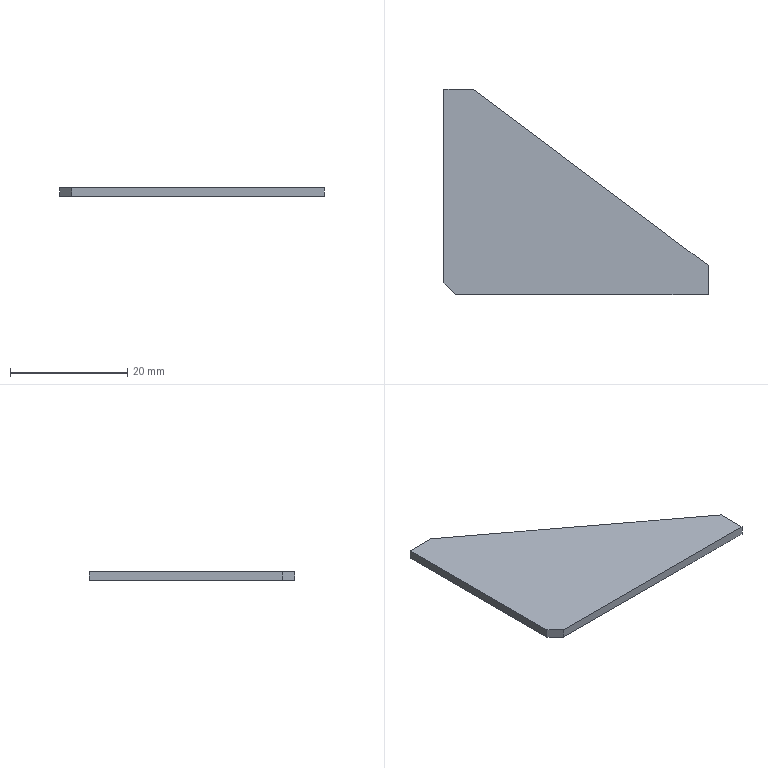Part | SolidWorks | features Extrusion 1 | 1 solid | 8 faces | box 45 x 35 x 1.5 mm | volume 1460 mm3 | plane 8
STEP:
#1=CARTESIAN_POINT('',(-20.5,-17.5,0.));
#2=VERTEX_POINT('',#1);
#3=CARTESIAN_POINT('',(22.5,-17.5,0.));
#4=VERTEX_POINT('',#3);
#5=CARTESIAN_POINT('',(22.5,-17.5,0.));
#6=DIRECTION('',(1.,0.,0.));
#7=VECTOR('',#6,1000.);
#8=LINE('',#5,#7);
#9=EDGE_CURVE('',#2,#4,#8,.T.);
#10=ORIENTED_EDGE('',*,*,#9,.T.);
#11=CARTESIAN_POINT('',(22.5,-17.5,1.5));
#12=VERTEX_POINT('',#11);
#13=CARTESIAN_POINT('',(22.5,-17.5,1.5));
#14=DIRECTION('',(0.,0.,-1.));
#15=VECTOR('',#14,1000.);
#16=LINE('',#13,#15);
#17=EDGE_CURVE('',#12,#4,#16,.T.);
#18=ORIENTED_EDGE('',*,*,#17,.F.);
#19=CARTESIAN_POINT('',(-20.5,-17.5,1.5));
#20=VERTEX_POINT('',#19);
#21=CARTESIAN_POINT('',(22.5,-17.5,1.5));
#22=DIRECTION('',(1.,0.,0.));
#23=VECTOR('',#22,1000.);
#24=LINE('',#21,#23);
#25=EDGE_CURVE('',#20,#12,#24,.T.);
#26=ORIENTED_EDGE('',*,*,#25,.F.);
#27=CARTESIAN_POINT('',(-20.5,-17.5,1.5));
#28=DIRECTION('',(0.,0.,-1.));
#29=VECTOR('',#28,1000.);
#30=LINE('',#27,#29);
#31=EDGE_CURVE('',#20,#2,#30,.T.);
#32=ORIENTED_EDGE('',*,*,#31,.T.);
#33=EDGE_LOOP('',(#10,#18,#26,#32));
#34=FACE_OUTER_BOUND('',#33,.T.);
#35=CARTESIAN_POINT('',(22.5,-17.5,1.5));
#36=DIRECTION('',(0.,1.,0.));
#37=DIRECTION('',(-1.,0.,0.));
#38=AXIS2_PLACEMENT_3D('',#35,#36,#37);
#39=PLANE('',#38);
#40=ADVANCED_FACE('',(#34),#39,.F.);
#41=CARTESIAN_POINT('',(22.5,-12.5,0.));
#42=VERTEX_POINT('',#41);
#43=CARTESIAN_POINT('',(22.5,-12.5,0.));
#44=DIRECTION('',(0.,1.,0.));
#45=VECTOR('',#44,1000.);
#46=LINE('',#43,#45);
#47=EDGE_CURVE('',#4,#42,#46,.T.);
#48=ORIENTED_EDGE('',*,*,#47,.T.);
#49=CARTESIAN_POINT('',(22.5,-12.5,1.5));
#50=VERTEX_POINT('',#49);
#51=CARTESIAN_POINT('',(22.5,-12.5,1.5));
#52=DIRECTION('',(0.,0.,-1.));
#53=VECTOR('',#52,1000.);
#54=LINE('',#51,#53);
#55=EDGE_CURVE('',#50,#42,#54,.T.);
#56=ORIENTED_EDGE('',*,*,#55,.F.);
#57=CARTESIAN_POINT('',(22.5,-12.5,1.5));
#58=DIRECTION('',(0.,1.,0.));
#59=VECTOR('',#58,1000.);
#60=LINE('',#57,#59);
#61=EDGE_CURVE('',#12,#50,#60,.T.);
#62=ORIENTED_EDGE('',*,*,#61,.F.);
#63=ORIENTED_EDGE('',*,*,#17,.T.);
#64=EDGE_LOOP('',(#48,#56,#62,#63));
#65=FACE_OUTER_BOUND('',#64,.T.);
#66=CARTESIAN_POINT('',(22.5,-12.5,1.5));
#67=DIRECTION('',(-1.,0.,0.));
#68=DIRECTION('',(0.,0.,1.));
#69=AXIS2_PLACEMENT_3D('',#66,#67,#68);
#70=PLANE('',#69);
#71=ADVANCED_FACE('',(#65),#70,.F.);
#72=CARTESIAN_POINT('',(-17.5,17.5,0.));
#73=VERTEX_POINT('',#72);
#74=CARTESIAN_POINT('',(-17.5,17.5,0.));
#75=DIRECTION('',(-0.8,0.6,0.));
#76=VECTOR('',#75,1000.);
#77=LINE('',#74,#76);
#78=EDGE_CURVE('',#42,#73,#77,.T.);
#79=ORIENTED_EDGE('',*,*,#78,.T.);
#80=CARTESIAN_POINT('',(-17.5,17.5,1.5));
#81=VERTEX_POINT('',#80);
#82=CARTESIAN_POINT('',(-17.5,17.5,1.5));
#83=DIRECTION('',(0.,0.,-1.));
#84=VECTOR('',#83,1000.);
#85=LINE('',#82,#84);
#86=EDGE_CURVE('',#81,#73,#85,.T.);
#87=ORIENTED_EDGE('',*,*,#86,.F.);
#88=CARTESIAN_POINT('',(-17.5,17.5,1.5));
#89=DIRECTION('',(-0.8,0.6,0.));
#90=VECTOR('',#89,1000.);
#91=LINE('',#88,#90);
#92=EDGE_CURVE('',#50,#81,#91,.T.);
#93=ORIENTED_EDGE('',*,*,#92,.F.);
#94=ORIENTED_EDGE('',*,*,#55,.T.);
#95=EDGE_LOOP('',(#79,#87,#93,#94));
#96=FACE_OUTER_BOUND('',#95,.T.);
#97=CARTESIAN_POINT('',(-17.5,17.5,1.5));
#98=DIRECTION('',(-0.6,-0.8,0.));
#99=DIRECTION('',(0.8,-0.6,0.));
#100=AXIS2_PLACEMENT_3D('',#97,#98,#99);
#101=PLANE('',#100);
#102=ADVANCED_FACE('',(#96),#101,.F.);
#103=CARTESIAN_POINT('',(-22.5,17.5,0.));
#104=VERTEX_POINT('',#103);
#105=CARTESIAN_POINT('',(-17.5,17.5,0.));
#106=DIRECTION('',(-1.,0.,0.));
#107=VECTOR('',#106,1000.);
#108=LINE('',#105,#107);
#109=EDGE_CURVE('',#73,#104,#108,.T.);
#110=ORIENTED_EDGE('',*,*,#109,.T.);
#111=CARTESIAN_POINT('',(-22.5,17.5,1.5));
#112=VERTEX_POINT('',#111);
#113=CARTESIAN_POINT('',(-22.5,17.5,1.5));
#114=DIRECTION('',(0.,0.,-1.));
#115=VECTOR('',#114,1000.);
#116=LINE('',#113,#115);
#117=EDGE_CURVE('',#112,#104,#116,.T.);
#118=ORIENTED_EDGE('',*,*,#117,.F.);
#119=CARTESIAN_POINT('',(-17.5,17.5,1.5));
#120=DIRECTION('',(-1.,0.,0.));
#121=VECTOR('',#120,1000.);
#122=LINE('',#119,#121);
#123=EDGE_CURVE('',#81,#112,#122,.T.);
#124=ORIENTED_EDGE('',*,*,#123,.F.);
#125=ORIENTED_EDGE('',*,*,#86,.T.);
#126=EDGE_LOOP('',(#110,#118,#124,#125));
#127=FACE_OUTER_BOUND('',#126,.T.);
#128=CARTESIAN_POINT('',(-17.5,17.5,1.5));
#129=DIRECTION('',(0.,-1.,0.));
#130=DIRECTION('',(0.,0.,-1.));
#131=AXIS2_PLACEMENT_3D('',#128,#129,#130);
#132=PLANE('',#131);
#133=ADVANCED_FACE('',(#127),#132,.F.);
#134=CARTESIAN_POINT('',(-22.5,-15.5,0.));
#135=VERTEX_POINT('',#134);
#136=CARTESIAN_POINT('',(-22.5,17.5,0.));
#137=DIRECTION('',(0.,-1.,0.));
#138=VECTOR('',#137,1000.);
#139=LINE('',#136,#138);
#140=EDGE_CURVE('',#104,#135,#139,.T.);
#141=ORIENTED_EDGE('',*,*,#140,.T.);
#142=CARTESIAN_POINT('',(-22.5,-15.5,1.5));
#143=VERTEX_POINT('',#142);
#144=CARTESIAN_POINT('',(-22.5,-15.5,1.5));
#145=DIRECTION('',(0.,0.,-1.));
#146=VECTOR('',#145,1000.);
#147=LINE('',#144,#146);
#148=EDGE_CURVE('',#143,#135,#147,.T.);
#149=ORIENTED_EDGE('',*,*,#148,.F.);
#150=CARTESIAN_POINT('',(-22.5,17.5,1.5));
#151=DIRECTION('',(0.,-1.,0.));
#152=VECTOR('',#151,1000.);
#153=LINE('',#150,#152);
#154=EDGE_CURVE('',#112,#143,#153,.T.);
#155=ORIENTED_EDGE('',*,*,#154,.F.);
#156=ORIENTED_EDGE('',*,*,#117,.T.);
#157=EDGE_LOOP('',(#141,#149,#155,#156));
#158=FACE_OUTER_BOUND('',#157,.T.);
#159=CARTESIAN_POINT('',(-22.5,17.5,1.5));
#160=DIRECTION('',(1.,0.,0.));
#161=DIRECTION('',(0.,1.,0.));
#162=AXIS2_PLACEMENT_3D('',#159,#160,#161);
#163=PLANE('',#162);
#164=ADVANCED_FACE('',(#158),#163,.F.);
#165=CARTESIAN_POINT('',(-20.5,-17.5,0.));
#166=DIRECTION('',(0.7071,-0.7071,0.));
#167=VECTOR('',#166,1000.);
#168=LINE('',#165,#167);
#169=EDGE_CURVE('',#135,#2,#168,.T.);
#170=ORIENTED_EDGE('',*,*,#169,.T.);
#171=ORIENTED_EDGE('',*,*,#31,.F.);
#172=CARTESIAN_POINT('',(-20.5,-17.5,1.5));
#173=DIRECTION('',(0.7071,-0.7071,0.));
#174=VECTOR('',#173,1000.);
#175=LINE('',#172,#174);
#176=EDGE_CURVE('',#143,#20,#175,.T.);
#177=ORIENTED_EDGE('',*,*,#176,.F.);
#178=ORIENTED_EDGE('',*,*,#148,.T.);
#179=EDGE_LOOP('',(#170,#171,#177,#178));
#180=FACE_OUTER_BOUND('',#179,.T.);
#181=CARTESIAN_POINT('',(-20.5,-17.5,1.5));
#182=DIRECTION('',(0.7071,0.7071,0.));
#183=DIRECTION('',(-0.7071,0.7071,0.));
#184=AXIS2_PLACEMENT_3D('',#181,#182,#183);
#185=PLANE('',#184);
#186=ADVANCED_FACE('',(#180),#185,.F.);
#187=ORIENTED_EDGE('',*,*,#25,.T.);
#188=ORIENTED_EDGE('',*,*,#61,.T.);
#189=ORIENTED_EDGE('',*,*,#92,.T.);
#190=ORIENTED_EDGE('',*,*,#123,.T.);
#191=ORIENTED_EDGE('',*,*,#154,.T.);
#192=ORIENTED_EDGE('',*,*,#176,.T.);
#193=EDGE_LOOP('',(#187,#188,#189,#190,#191,#192));
#194=FACE_OUTER_BOUND('',#193,.T.);
#195=CARTESIAN_POINT('',(0.,0.,1.5));
#196=DIRECTION('',(0.,0.,1.));
#197=DIRECTION('',(1.,0.,0.));
#198=AXIS2_PLACEMENT_3D('',#195,#196,#197);
#199=PLANE('',#198);
#200=ADVANCED_FACE('',(#194),#199,.T.);
#201=ORIENTED_EDGE('',*,*,#9,.F.);
#202=ORIENTED_EDGE('',*,*,#169,.F.);
#203=ORIENTED_EDGE('',*,*,#140,.F.);
#204=ORIENTED_EDGE('',*,*,#109,.F.);
#205=ORIENTED_EDGE('',*,*,#78,.F.);
#206=ORIENTED_EDGE('',*,*,#47,.F.);
#207=EDGE_LOOP('',(#201,#202,#203,#204,#205,#206));
#208=FACE_OUTER_BOUND('',#207,.T.);
#209=CARTESIAN_POINT('',(0.,0.,0.));
#210=DIRECTION('',(0.,0.,1.));
#211=DIRECTION('',(1.,0.,0.));
#212=AXIS2_PLACEMENT_3D('',#209,#210,#211);
#213=PLANE('',#212);
#214=ADVANCED_FACE('',(#208),#213,.F.);
#215=CLOSED_SHELL('',(#40,#71,#102,#133,#164,#186,#200,#214));
#216=MANIFOLD_SOLID_BREP('',#215);
#217=CARTESIAN_POINT('',(0.,0.,0.));
#218=DIRECTION('',(0.,0.,1.));
#219=DIRECTION('',(1.,0.,0.));
#220=AXIS2_PLACEMENT_3D('',#217,#218,#219);
#221=(LENGTH_UNIT()NAMED_UNIT(*)SI_UNIT(.MILLI.,.METRE.));
#222=UNCERTAINTY_MEASURE_WITH_UNIT(LENGTH_MEASURE(0.00001),#221,'','');
#223=(NAMED_UNIT(*)PLANE_ANGLE_UNIT()SI_UNIT($,.RADIAN.));
#224=(NAMED_UNIT(*)SI_UNIT($,.STERADIAN.)SOLID_ANGLE_UNIT());
#225=(GEOMETRIC_REPRESENTATION_CONTEXT(3)GLOBAL_UNCERTAINTY_ASSIGNED_CONTEXT((#222))GLOBAL_UNIT_ASSIGNED_CONTEXT((#221,#223,#224))REPRESENTATION_CONTEXT('',''));
#226=ADVANCED_BREP_SHAPE_REPRESENTATION('',(#216,#220),#225);